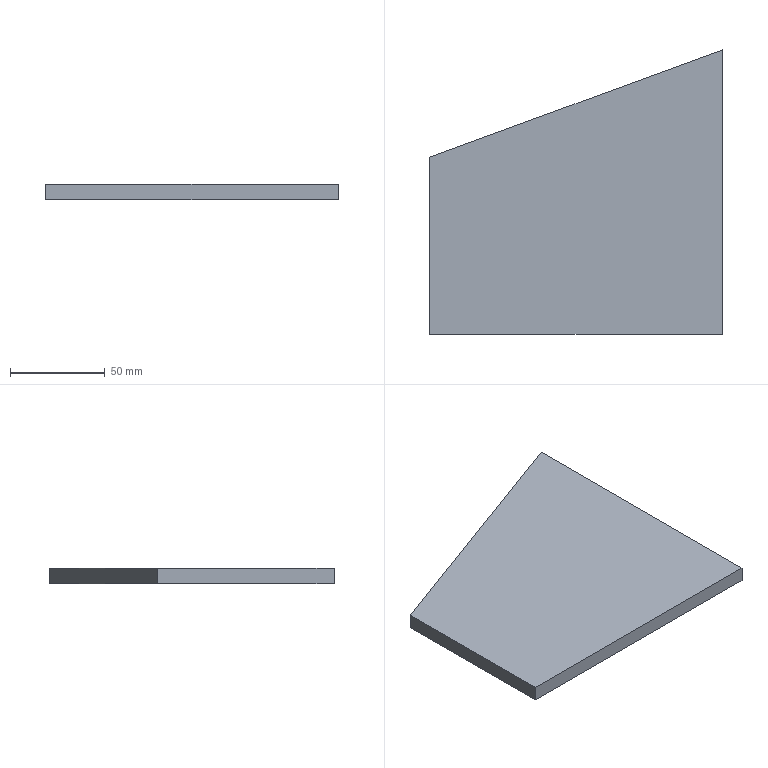Part | SolidWorks | features Extrusion 1 | 1 solid | 6 faces | box 154.478 x 150 x 8 mm | volume 150374 mm3 | plane 6
STEP:
#1=CARTESIAN_POINT('',(184.478,193.,0.));
#2=VERTEX_POINT('',#1);
#3=CARTESIAN_POINT('',(338.956,193.,0.));
#4=VERTEX_POINT('',#3);
#5=CARTESIAN_POINT('',(338.956,193.,0.));
#6=DIRECTION('',(1.,0.,0.));
#7=VECTOR('',#6,1000.);
#8=LINE('',#5,#7);
#9=EDGE_CURVE('',#2,#4,#8,.T.);
#10=ORIENTED_EDGE('',*,*,#9,.T.);
#11=CARTESIAN_POINT('',(338.956,193.,8.));
#12=VERTEX_POINT('',#11);
#13=CARTESIAN_POINT('',(338.956,193.,8.));
#14=DIRECTION('',(0.,0.,-1.));
#15=VECTOR('',#14,1000.);
#16=LINE('',#13,#15);
#17=EDGE_CURVE('',#12,#4,#16,.T.);
#18=ORIENTED_EDGE('',*,*,#17,.F.);
#19=CARTESIAN_POINT('',(184.478,193.,8.));
#20=VERTEX_POINT('',#19);
#21=CARTESIAN_POINT('',(338.956,193.,8.));
#22=DIRECTION('',(1.,0.,0.));
#23=VECTOR('',#22,1000.);
#24=LINE('',#21,#23);
#25=EDGE_CURVE('',#20,#12,#24,.T.);
#26=ORIENTED_EDGE('',*,*,#25,.F.);
#27=CARTESIAN_POINT('',(184.478,193.,8.));
#28=DIRECTION('',(0.,0.,-1.));
#29=VECTOR('',#28,1000.);
#30=LINE('',#27,#29);
#31=EDGE_CURVE('',#20,#2,#30,.T.);
#32=ORIENTED_EDGE('',*,*,#31,.T.);
#33=EDGE_LOOP('',(#10,#18,#26,#32));
#34=FACE_OUTER_BOUND('',#33,.T.);
#35=CARTESIAN_POINT('',(338.956,193.,8.));
#36=DIRECTION('',(0.,1.,0.));
#37=DIRECTION('',(-1.,0.,0.));
#38=AXIS2_PLACEMENT_3D('',#35,#36,#37);
#39=PLANE('',#38);
#40=ADVANCED_FACE('',(#34),#39,.F.);
#41=CARTESIAN_POINT('',(338.956,343.,0.));
#42=VERTEX_POINT('',#41);
#43=CARTESIAN_POINT('',(338.956,343.,0.));
#44=DIRECTION('',(0.,1.,0.));
#45=VECTOR('',#44,1000.);
#46=LINE('',#43,#45);
#47=EDGE_CURVE('',#4,#42,#46,.T.);
#48=ORIENTED_EDGE('',*,*,#47,.T.);
#49=CARTESIAN_POINT('',(338.956,343.,8.));
#50=VERTEX_POINT('',#49);
#51=CARTESIAN_POINT('',(338.956,343.,8.));
#52=DIRECTION('',(0.,0.,-1.));
#53=VECTOR('',#52,1000.);
#54=LINE('',#51,#53);
#55=EDGE_CURVE('',#50,#42,#54,.T.);
#56=ORIENTED_EDGE('',*,*,#55,.F.);
#57=CARTESIAN_POINT('',(338.956,343.,8.));
#58=DIRECTION('',(0.,1.,0.));
#59=VECTOR('',#58,1000.);
#60=LINE('',#57,#59);
#61=EDGE_CURVE('',#12,#50,#60,.T.);
#62=ORIENTED_EDGE('',*,*,#61,.F.);
#63=ORIENTED_EDGE('',*,*,#17,.T.);
#64=EDGE_LOOP('',(#48,#56,#62,#63));
#65=FACE_OUTER_BOUND('',#64,.T.);
#66=CARTESIAN_POINT('',(338.956,343.,8.));
#67=DIRECTION('',(-1.,0.,0.));
#68=DIRECTION('',(0.,0.,1.));
#69=AXIS2_PLACEMENT_3D('',#66,#67,#68);
#70=PLANE('',#69);
#71=ADVANCED_FACE('',(#65),#70,.F.);
#72=CARTESIAN_POINT('',(184.478,286.358,0.));
#73=VERTEX_POINT('',#72);
#74=CARTESIAN_POINT('',(184.478,286.358,0.));
#75=DIRECTION('',(-0.9389,-0.3443,0.));
#76=VECTOR('',#75,1000.);
#77=LINE('',#74,#76);
#78=EDGE_CURVE('',#42,#73,#77,.T.);
#79=ORIENTED_EDGE('',*,*,#78,.T.);
#80=CARTESIAN_POINT('',(184.478,286.358,8.));
#81=VERTEX_POINT('',#80);
#82=CARTESIAN_POINT('',(184.478,286.358,8.));
#83=DIRECTION('',(0.,0.,-1.));
#84=VECTOR('',#83,1000.);
#85=LINE('',#82,#84);
#86=EDGE_CURVE('',#81,#73,#85,.T.);
#87=ORIENTED_EDGE('',*,*,#86,.F.);
#88=CARTESIAN_POINT('',(184.478,286.358,8.));
#89=DIRECTION('',(-0.9389,-0.3443,0.));
#90=VECTOR('',#89,1000.);
#91=LINE('',#88,#90);
#92=EDGE_CURVE('',#50,#81,#91,.T.);
#93=ORIENTED_EDGE('',*,*,#92,.F.);
#94=ORIENTED_EDGE('',*,*,#55,.T.);
#95=EDGE_LOOP('',(#79,#87,#93,#94));
#96=FACE_OUTER_BOUND('',#95,.T.);
#97=CARTESIAN_POINT('',(184.478,286.358,8.));
#98=DIRECTION('',(0.3443,-0.9389,0.));
#99=DIRECTION('',(0.9389,0.3443,0.));
#100=AXIS2_PLACEMENT_3D('',#97,#98,#99);
#101=PLANE('',#100);
#102=ADVANCED_FACE('',(#96),#101,.F.);
#103=CARTESIAN_POINT('',(184.478,193.,0.));
#104=DIRECTION('',(0.,-1.,0.));
#105=VECTOR('',#104,1000.);
#106=LINE('',#103,#105);
#107=EDGE_CURVE('',#73,#2,#106,.T.);
#108=ORIENTED_EDGE('',*,*,#107,.T.);
#109=ORIENTED_EDGE('',*,*,#31,.F.);
#110=CARTESIAN_POINT('',(184.478,193.,8.));
#111=DIRECTION('',(0.,-1.,0.));
#112=VECTOR('',#111,1000.);
#113=LINE('',#110,#112);
#114=EDGE_CURVE('',#81,#20,#113,.T.);
#115=ORIENTED_EDGE('',*,*,#114,.F.);
#116=ORIENTED_EDGE('',*,*,#86,.T.);
#117=EDGE_LOOP('',(#108,#109,#115,#116));
#118=FACE_OUTER_BOUND('',#117,.T.);
#119=CARTESIAN_POINT('',(184.478,193.,8.));
#120=DIRECTION('',(1.,0.,0.));
#121=DIRECTION('',(0.,1.,0.));
#122=AXIS2_PLACEMENT_3D('',#119,#120,#121);
#123=PLANE('',#122);
#124=ADVANCED_FACE('',(#118),#123,.F.);
#125=ORIENTED_EDGE('',*,*,#25,.T.);
#126=ORIENTED_EDGE('',*,*,#61,.T.);
#127=ORIENTED_EDGE('',*,*,#92,.T.);
#128=ORIENTED_EDGE('',*,*,#114,.T.);
#129=EDGE_LOOP('',(#125,#126,#127,#128));
#130=FACE_OUTER_BOUND('',#129,.T.);
#131=CARTESIAN_POINT('',(0.,0.,8.));
#132=DIRECTION('',(0.,0.,-1.));
#133=DIRECTION('',(-1.,0.,0.));
#134=AXIS2_PLACEMENT_3D('',#131,#132,#133);
#135=PLANE('',#134);
#136=ADVANCED_FACE('',(#130),#135,.F.);
#137=ORIENTED_EDGE('',*,*,#9,.F.);
#138=ORIENTED_EDGE('',*,*,#107,.F.);
#139=ORIENTED_EDGE('',*,*,#78,.F.);
#140=ORIENTED_EDGE('',*,*,#47,.F.);
#141=EDGE_LOOP('',(#137,#138,#139,#140));
#142=FACE_OUTER_BOUND('',#141,.T.);
#143=CARTESIAN_POINT('',(0.,0.,0.));
#144=DIRECTION('',(0.,0.,-1.));
#145=DIRECTION('',(-1.,0.,0.));
#146=AXIS2_PLACEMENT_3D('',#143,#144,#145);
#147=PLANE('',#146);
#148=ADVANCED_FACE('',(#142),#147,.T.);
#149=CLOSED_SHELL('',(#40,#71,#102,#124,#136,#148));
#150=MANIFOLD_SOLID_BREP('',#149);
#151=CARTESIAN_POINT('',(0.,0.,0.));
#152=DIRECTION('',(0.,0.,1.));
#153=DIRECTION('',(1.,0.,0.));
#154=AXIS2_PLACEMENT_3D('',#151,#152,#153);
#155=(LENGTH_UNIT()NAMED_UNIT(*)SI_UNIT(.MILLI.,.METRE.));
#156=UNCERTAINTY_MEASURE_WITH_UNIT(LENGTH_MEASURE(0.00001),#155,'','');
#157=(NAMED_UNIT(*)PLANE_ANGLE_UNIT()SI_UNIT($,.RADIAN.));
#158=(NAMED_UNIT(*)SI_UNIT($,.STERADIAN.)SOLID_ANGLE_UNIT());
#159=(GEOMETRIC_REPRESENTATION_CONTEXT(3)GLOBAL_UNCERTAINTY_ASSIGNED_CONTEXT((#156))GLOBAL_UNIT_ASSIGNED_CONTEXT((#155,#157,#158))REPRESENTATION_CONTEXT('',''));
#160=ADVANCED_BREP_SHAPE_REPRESENTATION('',(#150,#154),#159);